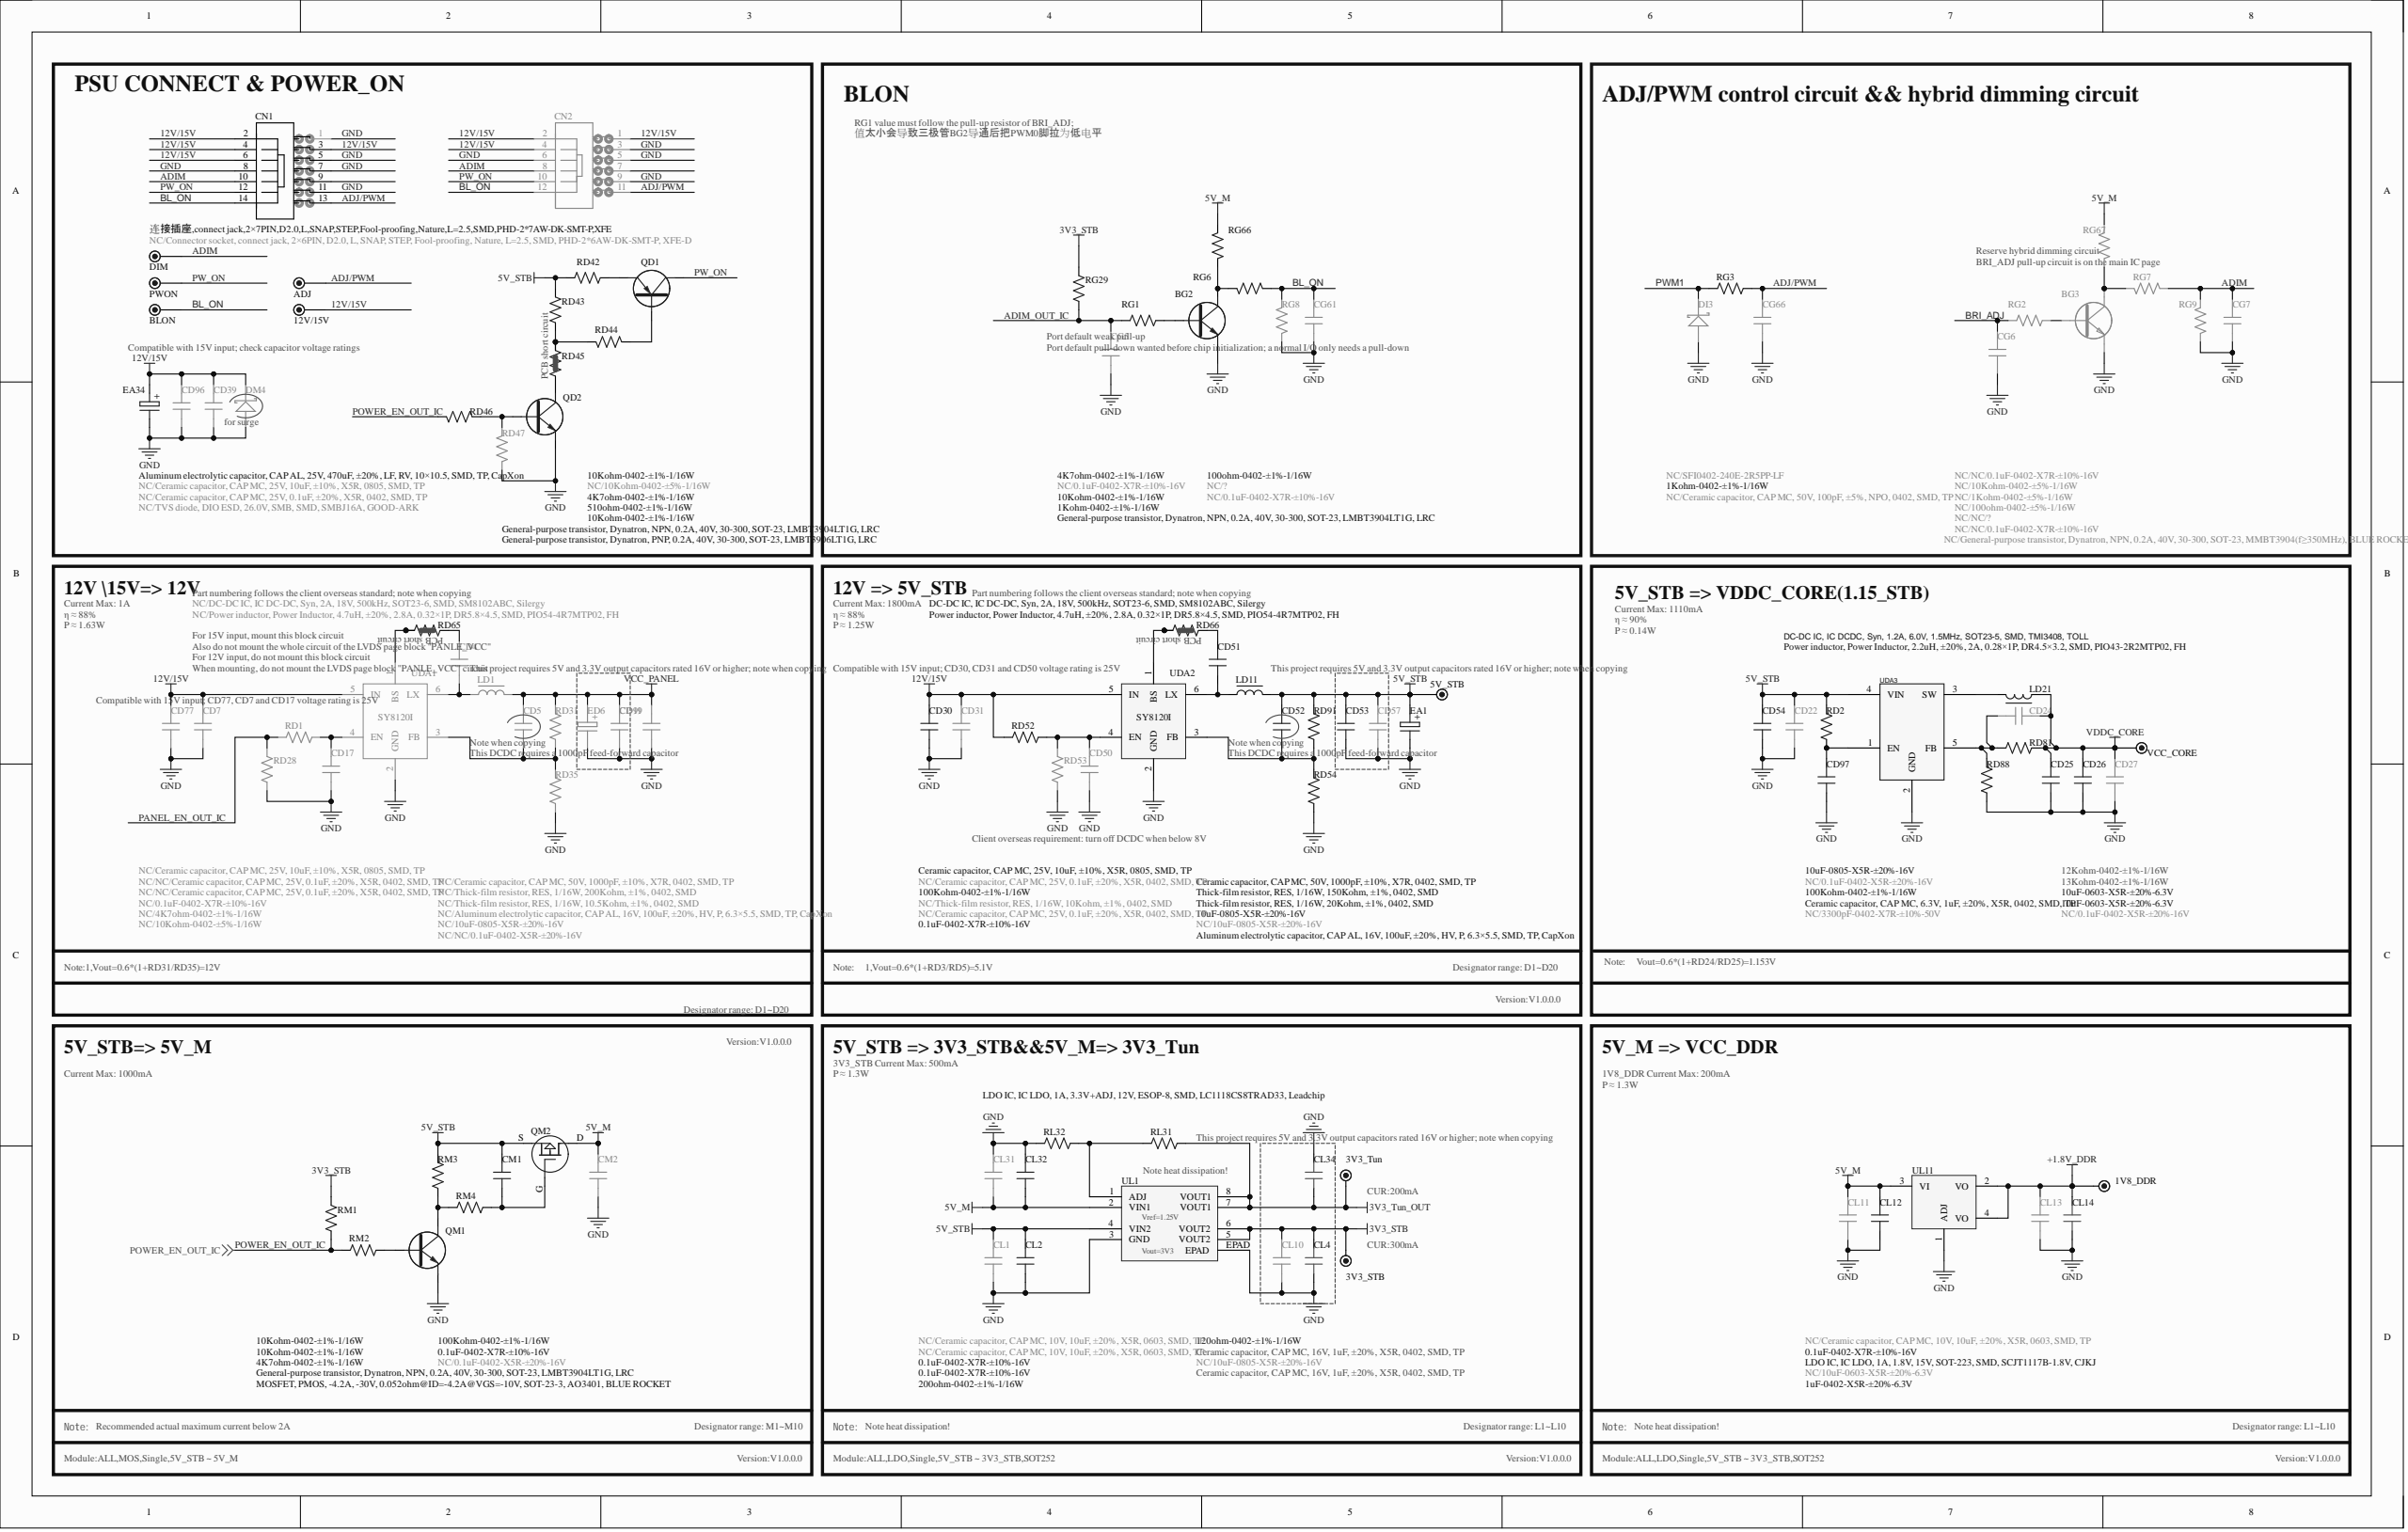Circuit board | Altium Designer | 541 parts | 263 nets | one sheet of the schematic
Parts on this sheet (reference | value | footprint):
1V8_DDR | TEST | TP
ADJ | TEST | TP
BG2 | General-purpose transistor, Dynatron, NPN, 0.2A, 40V, 30-300, SOT-23, LMBT3904LT1G, LRC | SOT-23
BG3 | NC/General-purpose transistor, Dynatron, NPN, 0.2A, 40V, 30-300, SOT-23, MMBT3904(f=350MHz), BLUE ROCKET | SOT-23
BLON | TEST | TP
CD4 | NC/0.1uF-0402-X7R-±10%-16V | C0402
CD5 | NC/Ceramic capacitor, CAP MC, 50V, 1000pF, ±10%, X7R, 0402, SMD, TP | C0402
CD7 | NC/NC/Ceramic capacitor, CAP MC, 25V, 0.1uF, ±20%, X5R, 0402, SMD, TP | C0402
CD11 | NC/NC/0.1uF-0402-X5R-±20%-16V | C0402
CD17 | NC/NC/Ceramic capacitor, CAP MC, 25V, 0.1uF, ±20%, X5R, 0402, SMD, TP | C0402
CD22 | NC/0.1uF-0402-X5R-±20%-16V | C0402
CD24 | NC/3300pF-0402-X7R-±10%-50V | C0402
CD25 | 10uF-0603-X5R-±20%-6.3V | C0603
CD26 | 10uF-0603-X5R-±20%-6.3V | C0603
CD27 | NC/0.1uF-0402-X5R-±20%-16V | C0402
CD30 | Ceramic capacitor, CAP MC, 25V, 10uF, ±10%, X5R, 0805, SMD, TP | C0805
CD31 | NC/Ceramic capacitor, CAP MC, 25V, 0.1uF, ±20%, X5R, 0402, SMD, TP | C0402
CD39 | NC/Ceramic capacitor, CAP MC, 25V, 0.1uF, ±20%, X5R, 0402, SMD, TP | C0402
CD50 | NC/Ceramic capacitor, CAP MC, 25V, 0.1uF, ±20%, X5R, 0402, SMD, TP | C0402
CD51 | 0.1uF-0402-X7R-±10%-16V | C0402
CD52 | Ceramic capacitor, CAP MC, 50V, 1000pF, ±10%, X7R, 0402, SMD, TP | C0402
CD53 | 10uF-0805-X5R-±20%-16V | C0805
CD54 | 10uF-0805-X5R-±20%-16V | C0805
CD57 | NC/10uF-0805-X5R-±20%-16V | C0805
CD77 | NC/Ceramic capacitor, CAP MC, 25V, 10uF, ±10%, X5R, 0805, SMD, TP | C0805
CD96 | NC/Ceramic capacitor, CAP MC, 25V, 10uF, ±10%, X5R, 0805, SMD, TP | C0805
CD97 | Ceramic capacitor, CAP MC, 6.3V, 1uF, ±20%, X5R, 0402, SMD, TP | C0402
CD99 | NC/10uF-0805-X5R-±20%-16V | C0805
CG5 | NC/0.1uF-0402-X7R-±10%-16V | C0402
CG6 | NC/NC/0.1uF-0402-X7R-±10%-16V | C0402
CG7 | NC/NC/0.1uF-0402-X7R-±10%-16V | C0402
CG61 | NC/0.1uF-0402-X7R-±10%-16V | C0402
CG66 | NC/Ceramic capacitor, CAP MC, 50V, 100pF, ±5%, NPO, 0402, SMD, TP | C0402
CL1 | NC/Ceramic capacitor, CAP MC, 10V, 10uF, ±20%, X5R, 0603, SMD, TP | C0603
CL2 | 0.1uF-0402-X7R-±10%-16V | C0402
CL4 | Ceramic capacitor, CAP MC, 16V, 1uF, ±20%, X5R, 0402, SMD, TP | C0402
CL10 | NC/10uF-0805-X5R-±20%-16V | C0805
CL11 | NC/Ceramic capacitor, CAP MC, 10V, 10uF, ±20%, X5R, 0603, SMD, TP | C0603
CL12 | 0.1uF-0402-X7R-±10%-16V | C0402
CL13 | NC/10uF-0603-X5R-±20%-6.3V | C0603
CL14 | 1uF-0402-X5R-±20%-6.3V | C0402
CL31 | NC/Ceramic capacitor, CAP MC, 10V, 10uF, ±20%, X5R, 0603, SMD, TP | C0603
CL32 | 0.1uF-0402-X7R-±10%-16V | C0402
CL34 | Ceramic capacitor, CAP MC, 16V, 1uF, ±20%, X5R, 0402, SMD, TP | C0402
CM1 | 0.1uF-0402-X7R-±10%-16V | C0402
CM2 | NC/0.1uF-0402-X5R-±20%-16V | C0402
CN1 | 连接插座,connect jack,2×7PIN,D2.0,L,SNAP,STEP,Fool-proofing,Nature,L=2.5,SMD,PHD-2*7AW-DK-SMT-P,XFE | SIP2*7H/2.0D-LS
CN2 | NC/Connector socket, connect jack, 2×6PIN, D2.0, L, SNAP, STEP, Fool-proofing, Nature, L=2.5, SMD, PHD-2*6AW-DK-SMT-P, XFE-D | SIP2*6H/2.0D-LS
DI3 | NC/SFI0402-240E-2R5PP-LF | DIODE-S0402
DIM | TEST | TP
DM4 | NC/TVS diode, DIO ESD, 26.0V, SMB, SMD, SMBJ16A, GOOD-ARK | DIODE-SMB-2
EA34 | Aluminum electrolytic capacitor, CAP AL, 25V, 470uF, ±20%, LF, RV, 10×10.5, SMD, TP, CapXon | EC(10*10.5)-S
LD1 | NC/Power inductor, Power Inductor, 4.7uH, ±20%, 2.8A, 0.32×1P, DR5.8×4.5, SMD, PIO54-4R7MTP02, FH | L(5.8*4.5)-S
LD11 | Power inductor, Power Inductor, 4.7uH, ±20%, 2.8A, 0.32×1P, DR5.8×4.5, SMD, PIO54-4R7MTP02, FH | L(5.8*4.5)-S
LD21 | Power inductor, Power Inductor, 2.2uH, ±20%, 2A, 0.28×1P, DR4.5×3.2, SMD, PIO43-2R2MTP02, FH | L(4.5*3.5)-S
PWON | TEST | TP
QD1 | General-purpose transistor, Dynatron, PNP, 0.2A, 40V, 30-300, SOT-23, LMBT3906LT1G, LRC | SOT-23
QD2 | General-purpose transistor, Dynatron, NPN, 0.2A, 40V, 30-300, SOT-23, LMBT3904LT1G, LRC | SOT-23
QM1 | General-purpose transistor, Dynatron, NPN, 0.2A, 40V, 30-300, SOT-23, LMBT3904LT1G, LRC | SOT-23
QM2 | MOSFET, PMOS, -4.2A, -30V, 0.052ohm@ID=-4.2A@VGS=-10V, SOT-23-3, AO3401, BLUE ROCKET | SOT-23-1
RD1 | NC/10Kohm-0402-±5%-1/16W | R0402
RD2 | 100Kohm-0402-±1%-1/16W | R0402
RD28 | NC/4K7ohm-0402-±1%-1/16W | R0402
RD31 | NC/Thick-film resistor, RES, 1/16W, 200Kohm, ±1%, 0402, SMD | R0402
RD35 | NC/Thick-film resistor, RES, 1/16W, 10.5Kohm, ±1%, 0402, SMD | R0402
RD42 | 510ohm-0402-±1%-1/16W | R0402
RD43 | 4K7ohm-0402-±1%-1/16W | R0402
RD44 | 10Kohm-0402-±1%-1/16W | R0402
RD45 | NC/0ohm-0402-PCB | R0402SC
RD46 | 10Kohm-0402-±1%-1/16W | R0402
RD47 | NC/10Kohm-0402-±5%-1/16W | R0402
RD52 | 100Kohm-0402-±1%-1/16W | R0402
RD53 | NC/Thick-film resistor, RES, 1/16W, 10Kohm, ±1%, 0402, SMD | R0402
RD54 | Thick-film resistor, RES, 1/16W, 20Kohm, ±1%, 0402, SMD | R0402
RD65 | NC/0ohm-0402-PCB | R0402SC
RD66 | NC/0ohm-0402-PCB | R0402SC
RD81 | 12Kohm-0402-±1%-1/16W | R0402
RD88 | 13Kohm-0402-±1%-1/16W | R0402
RD91 | Thick-film resistor, RES, 1/16W, 150Kohm, ±1%, 0402, SMD | R0402
RG1 | 10Kohm-0402-±1%-1/16W | R0402
RG2 | NC/10Kohm-0402-±5%-1/16W | R0402
RG3 | 1Kohm-0402-±1%-1/16W | R0402
RG6 | 100ohm-0402-±1%-1/16W | R0402
RG7 | NC/100ohm-0402-±5%-1/16W | R0402
RG8 | NC/? | R0402
RG9 | NC/NC/? | R0402
RG29 | 4K7ohm-0402-±1%-1/16W | R0402
RG66 | 1Kohm-0402-±1%-1/16W | R0402
RG67 | NC/1Kohm-0402-±5%-1/16W | R0402
RL31 | 120ohm-0402-±1%-1/16W | R0402
RL32 | 200ohm-0402-±1%-1/16W | R0402
RM1 | 10Kohm-0402-±1%-1/16W | R0402
RM2 | 10Kohm-0402-±1%-1/16W | R0402
RM3 | 4K7ohm-0402-±1%-1/16W | R0402
RM4 | 100Kohm-0402-±1%-1/16W | R0402
UDA1 | NC/DC-DC IC, IC DC-DC, Syn, 2A, 18V, 500kHz, SOT23-6, SMD, SM8102ABC, Silergy | SOT23-6-2
UDA2 | DC-DC IC, IC DC-DC, Syn, 2A, 18V, 500kHz, SOT23-6, SMD, SM8102ABC, Silergy | SOT23-6-2
UDA3 | DC-DC IC, IC DCDC, Syn, 1.2A, 6.0V, 1.5MHz, SOT23-5, SMD, TMI3408, TOLL | SOT-23-5
UL1 | LDO IC, IC LDO, 1A, 3.3V+ADJ, 12V, ESOP-8, SMD, LC1118CS8TRAD33, Leadchip | SOP8/1.27-3
UL11 | LDO IC, IC LDO, 1A, 1.8V, 15V, SOT-223, SMD, SCJT1117B-1.8V, CJKJ | SOT-223
VCC_CORE | TEST | TP
Nets of these parts (net: part-pin ...):
VDDC_CORE: CD24-2 CD25-2 CD26-2 CD27-2 LD21-1 RD81-2 VCC_CORE-1
VCC_PANEL: CD5-2 CD11-2 CD99-1 LD1-2 RD31-2
PWM1: DI3-K RG3-2
PW_ON: CN1-12 CN2-10 PWON-1 QD1-C
POWER_EN_OUT_IC: RD46-1 RM1-1 RM2-1
PANEL_EN_OUT_IC: RD1-1 RD28-2
NetRL31_1: RL31-1 RL32-2 UL1-1
NetRD66_2: RD66-2 RD66-3 UDA2-1
NetRD65_2: RD65-2 RD65-3 UDA1-1
NetRD43_1: RD43-1 RD44-2 RD45-2 RD45-3
NetQM1_C: QM1-C RM3-1 RM4-1
NetQM1_B: QM1-B RM2-2
NetQD2_C: QD2-C RD45-1
NetQD2_B: QD2-B RD46-2 RD47-1
NetQD1_E: QD1-E RD42-1
NetQD1_B: QD1-B RD44-1
NetLD21_2: LD21-2 UDA3-3
NetCM1_1: CM1-1 QM2-G RM4-2
NetCD97_1: CD97-1 RD2-2 UDA3-1
NetCD52_1: CD52-1 RD54-2 RD91-1 UDA2-3
NetCD51_2: CD51-2 RD66-1
NetCD51_1: CD51-1 LD11-1 UDA2-6
NetCD50_1: CD50-1 RD52-2 RD53-1 UDA2-4
NetCD24_1: CD24-1 RD81-1 RD88-2 UDA3-5
NetCD17_1: CD17-1 RD1-2 UDA1-4
NetCD5_1: CD5-1 RD31-1 RD35-2 UDA1-3
NetCD4_2: CD4-2 RD65-1
NetCD4_1: CD4-1 LD1-1 UDA1-6
NetBG3_C: BG3-C RG7-2 RG67-1
NetBG3_B: BG3-B RG2-1
NetBG2_C: BG2-C RG6-2 RG66-1
NetBG2_B: BG2-B RG1-1
GND: BG2-E BG3-E CD7-2 CD11-1 CD17-2 CD22-1 CD25-1 CD26-1 CD27-1 CD30-1 CD31-2 CD39-2 CD50-2 CD53-2 CD54-2 CD57-2 CD77-1 CD96-1 CD97-2 CD99-2 CG5-1 CG6-1 CG7-1 CG61-1 CG66-1 CL1-1 CL2-1 CL4-2 CL10-2 CL11-1 CL12-1 CL13-1 CL14-1 CL31-2 CL32-2 CL34-1 CM2-1 CN1-1 CN1-5 CN1-7 CN1-8 CN1-11 CN2-3 CN2-5 CN2-6 CN2-9 DI3-A DM4-A EA34-2 QD2-E QM1-E RD28-1 RD35-1 RD47-2 RD53-2 RD54-1 RD88-1 RG8-1 RG9-1 RL32-1 UDA1-2 UDA2-2 UDA3-2 UL1-3 UL1-EPAD UL11-1
BRI_ADJ: CG6-2 RG2-2
BL_ON: BLON-1 CG61-2 CN1-14 CN2-12 RG6-1 RG8-2
ADJ/PWM: ADJ-1 CG66-2 CN1-13 CN2-11 RG3-1
ADIM_OUT_IC: CG5-2 RG1-2 RG29-1
ADIM: CG7-2 CN1-10 CN2-8 DIM-1 RG7-1 RG9-2
+1.8V_DDR: 1V8_DDR-1 CL13-2 CL14-2 UL11-2 UL11-4
12V/15V: CD7-1 CD30-2 CD31-1 CD39-1 CD77-2 CD96-2 CN1-2 CN1-3 CN1-4 CN1-6 CN2-1 CN2-2 CN2-4 DM4-K EA34-1 RD52-1 UDA1-5 UDA2-5
5V_STB: CD22-2 CD52-2 CD53-1 CD54-1 CD57-1 CL1-2 CL2-2 CM1-2 LD11-2 QM2-S RD2-1 RD42-2 RD43-2 RD91-2 RM3-2 UDA3-4 UL1-4
5V_M: CL11-2 CL12-2 CL31-1 CL32-1 CM2-2 QM2-D RG66-2 RG67-2 UL1-2 UL11-3
3V3_Tun_OUT: CL34-2 RL31-2 UL1-7 UL1-8
3V3_STB: CL4-1 CL10-1 RG29-2 RM1-2 UL1-5 UL1-6